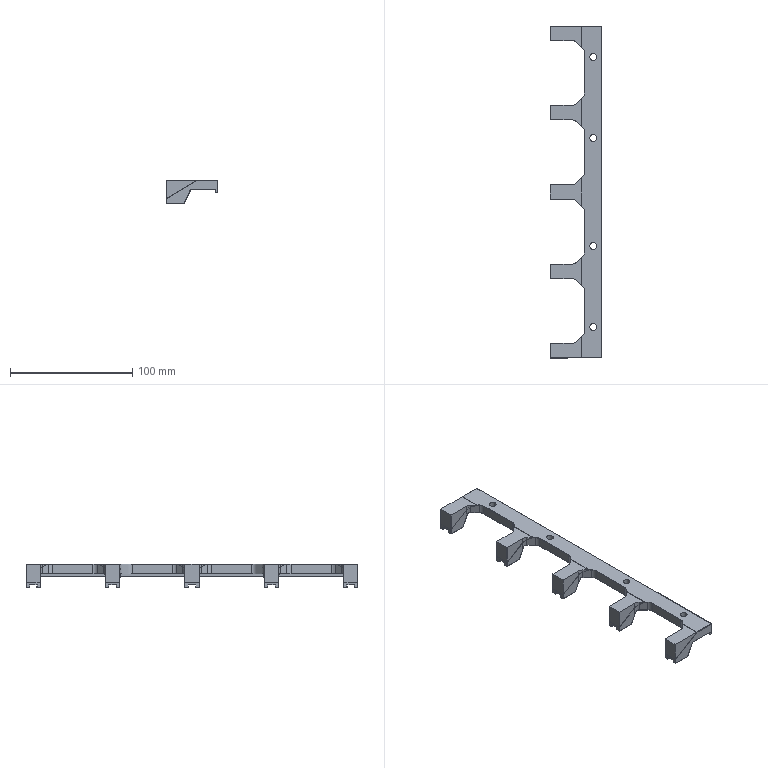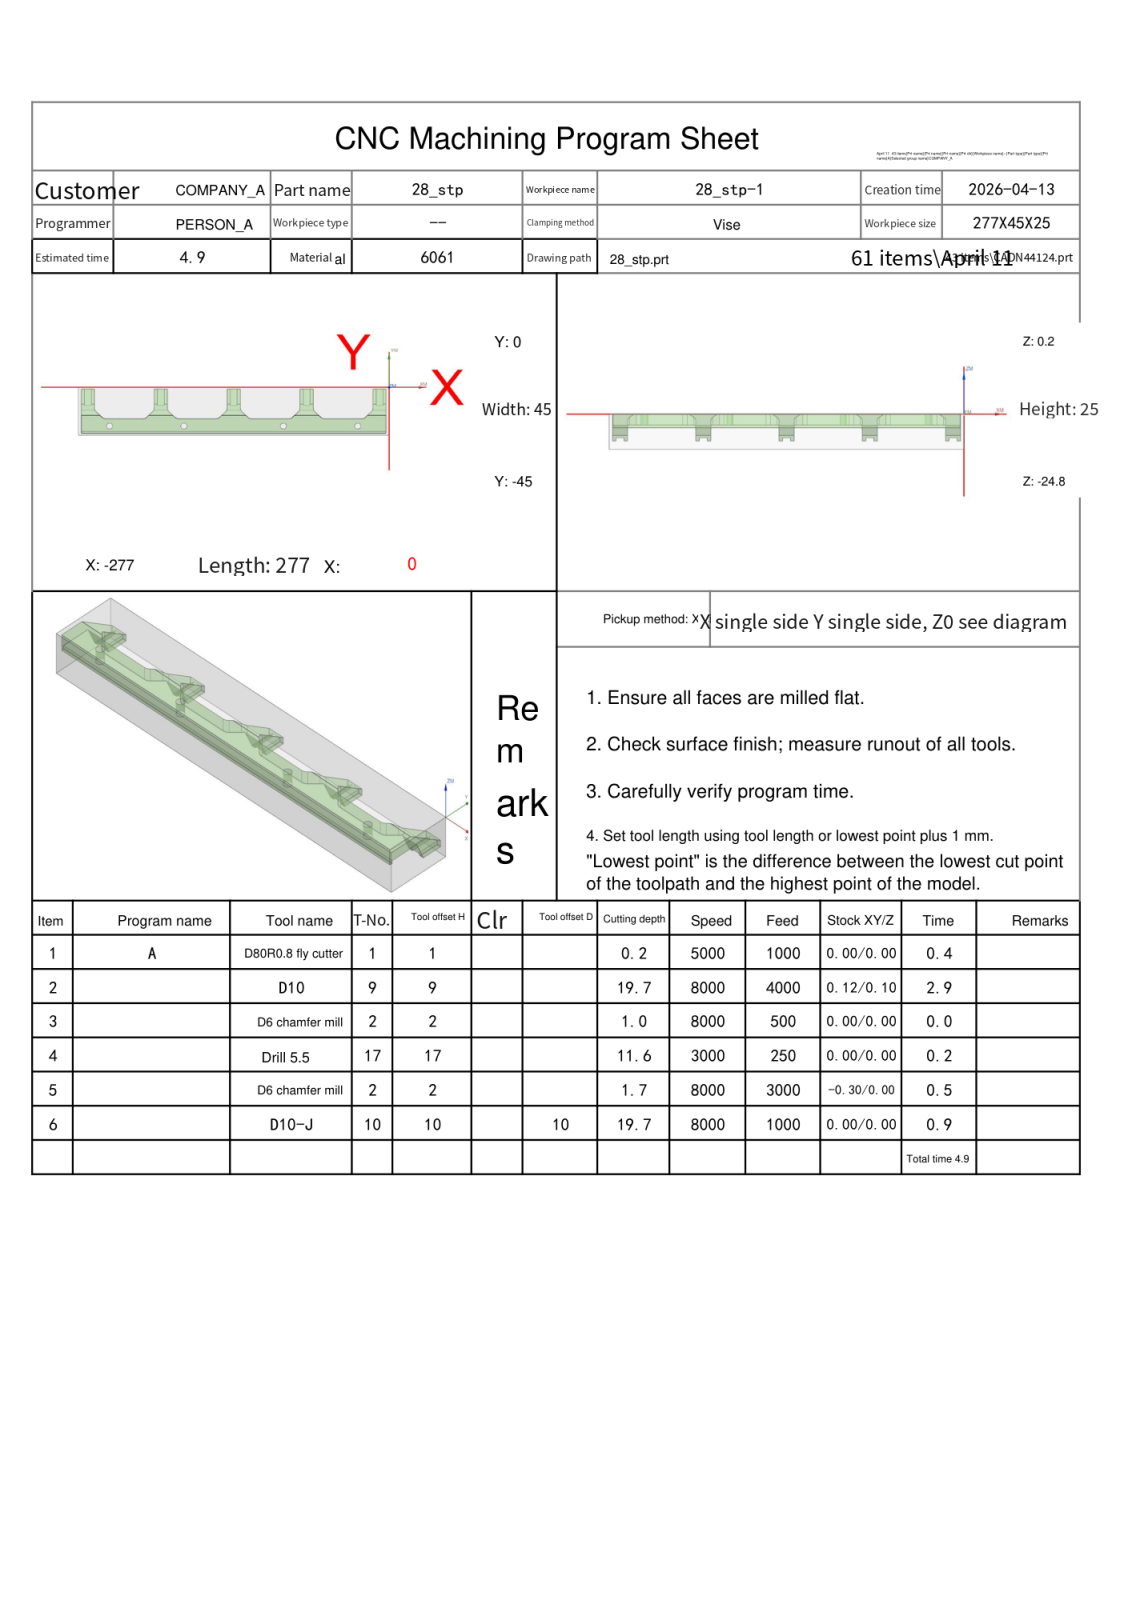NC program | NX | posted by the shop | part box 42 x 271.8 x 19 mm
Lines 1 to 31 of 2830:
%
O0001
(Machine time: 6.13 MIN)
(===Total Tool:5===)
(T1=D80R0.8 fly cutter D=80.  R=0.8  D-  H01 Z=-0.   )
(T9=D10     D=10.  R=0.   D-  H09 Z=-19.5 )
(T2=D6 chamfer mill   D=6.   R=0.   D-  H02 Z=-1.5  )
(T17=drill 5.5  D=5.5  DR_a=118 D-  H17 Z=-11.4 )
(T10=D10-J  D=10.  R=0.   D10 H10 Z=-19.5 )
G80 G90 G17 G49 G40
G91 G28 Z0
M01
N1 T01 M06
(D80R0.8 fly cutter  D=80. R=0.8 H=01 ce=0.00 di=0.00)
G00 G90 G54 X-319.4 Y-22.5 M03 S5000
G43 H01 Z20.
M08
Z2.
G01 Z0.0 F1000.
X-314.4
X37.4
X42.4
Z2.
G00 Z20.
G91 G28 Z0.0
M05
M09
G91 G28 Z0.0
M01